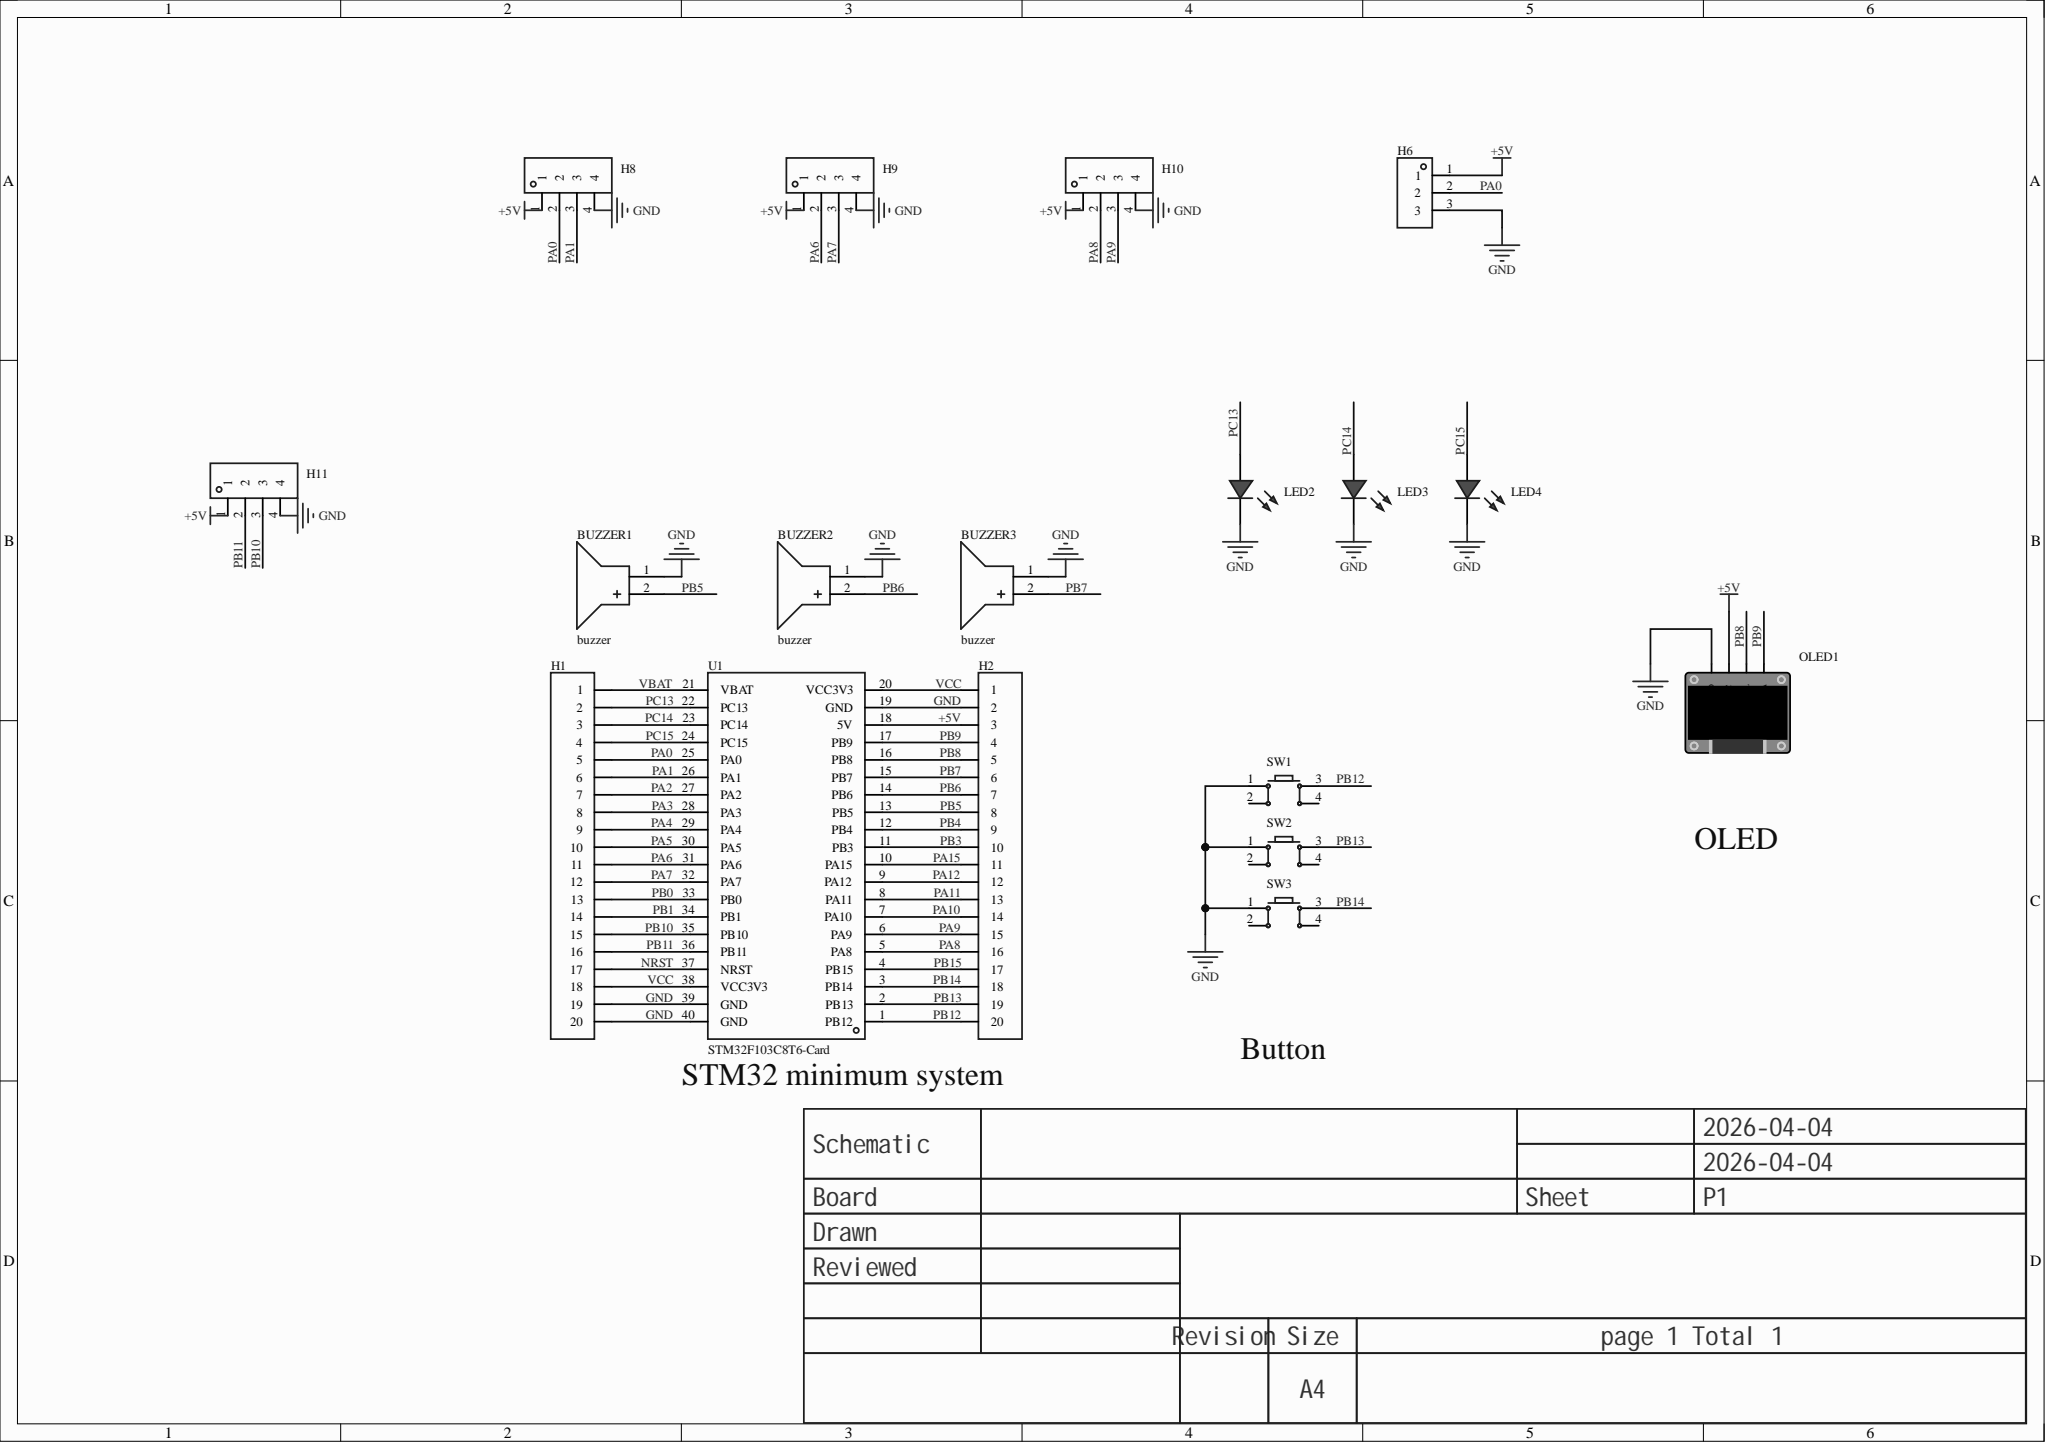Circuit board | Altium Designer | 18 parts | 37 nets
Bill of materials:
Comment,Description,Designator,Footprint,LibRef,Quantity
"buzzer","","BUZZER1, BUZZER2, BUZZER3","BUZ-TH_BD12.0-P6.00-D0.9-RD","buzzer","3"
"","","H1, H2","HDR-TH_20P-P2.54-V-F","HDR-F_2.54_1x20P","2"
"","","H6","HDR-TH_3P-P2.54-V-F","HDR-F_2.54_1x3P","1"
"","","H8, H9, H10, H11","HDR-TH_4P-P2.54-V-F","HDR-F_2.54_1x4P","4"
"","","LED2, LED3, LED4","LED-TH_5mm","LED_TH-R_5mm","3"
"","","OLED1","0.96OLED_4P","0.96OLED模块_4P","1"
"","","SW1, SW2, SW3","SW-TH_4P-L6.0-W6.0-P4.50-LS6.5","Key_TH_6x6x6","3"
"STM32F103C8T6-Card","","U1","CONN-TH_L53.3-W22.9_STM32F103C8T6-CARD","STM32F103C8T6-Card","1"
Netlist (Protel format):
[
BUZZER1
BUZ-TH_BD12.0-P6.00-D0.9-RD
buzzer



]
[
BUZZER2
BUZ-TH_BD12.0-P6.00-D0.9-RD
buzzer



]
[
BUZZER3
BUZ-TH_BD12.0-P6.00-D0.9-RD
buzzer



]
[
H1
HDR-TH_20P-P2.54-V-F




]
[
H2
HDR-TH_20P-P2.54-V-F




]
[
H6
HDR-TH_3P-P2.54-V-F




]
[
H8
HDR-TH_4P-P2.54-V-F




]
[
H9
HDR-TH_4P-P2.54-V-F




]
[
H10
HDR-TH_4P-P2.54-V-F




]
[
H11
HDR-TH_4P-P2.54-V-F




]
[
LED2
LED-TH_5mm




]
[
LED3
LED-TH_5mm




]
[
LED4
LED-TH_5mm




]
[
OLED1
0.96OLED_4P




]
[
SW1
SW-TH_4P-L6.0-W6.0-P4.50-LS6.5




]
[
SW2
SW-TH_4P-L6.0-W6.0-P4.50-LS6.5




]
[
SW3
SW-TH_4P-L6.0-W6.0-P4.50-LS6.5




]
[
U1
CONN-TH_L53.3-W22.9_STM32F103C8T6-CARD
STM32F103C8T6-Card



]
(
VCC
H1-18
H2-1
U1-20
U1-38
)
(
VBAT
H1-1
U1-21
)
(
PC15
H1-4
LED4-1
U1-24
)
(
PC14
H1-3
LED3-1
U1-23
)
(
PC13
H1-2
LED2-1
U1-22
)
(
PB15
H2-17
U1-4
)
(
PB14
H2-18
SW3-3
U1-3
)
(
PB13
H2-19
SW2-3
U1-2
)
(
PB12
H2-20
SW1-3
U1-1
)
(
PB11
H1-16
H11-2
U1-36
)
(
PB10
H1-15
H11-3
U1-35
)
(
PB9
H2-4
OLED1-4
U1-17
)
(
PB8
H2-5
OLED1-3
U1-16
)
(
PB7
BUZZER3-2
H2-6
U1-15
)
(
PB6
BUZZER2-2
H2-7
U1-14
)
(
PB5
BUZZER1-2
H2-8
U1-13
)
(
PB4
H2-9
U1-12
)
(
PB3
H2-10
U1-11
)
(
PB1
H1-14
U1-34
)
(
PB0
H1-13
U1-33
)
(
PA15
H2-11
U1-10
)
(
PA12
H2-12
U1-9
)
(
PA11
H2-13
U1-8
)
(
PA10
H2-14
U1-7
)
(
PA9
H2-15
H10-3
U1-6
)
(
PA8
H2-16
H10-2
U1-5
)
(
PA7
H1-12
H9-3
U1-32
)
(
PA6
H1-11
H9-2
U1-31
)
(
PA5
H1-10
U1-30
)
(
PA4
H1-9
U1-29
)
(
PA3
H1-8
U1-28
)
(
PA2
H1-7
U1-27
)
(
PA1
H1-6
H8-3
U1-26
)
(
PA0
H1-5
H6-2
H8-2
U1-25
)
(
NRST
H1-17
U1-37
)
(
GND
BUZZER1-1
BUZZER2-1
BUZZER3-1
H1-19
H1-20
H2-2
H6-3
H8-4
H9-4
H10-4
H11-4
LED2-2
LED3-2
LED4-2
OLED1-1
SW1-1
SW2-1
SW3-1
U1-19
U1-39
U1-40
)
(
+5V
H2-3
H6-1
H8-1
H9-1
H10-1
H11-1
OLED1-2
U1-18
)